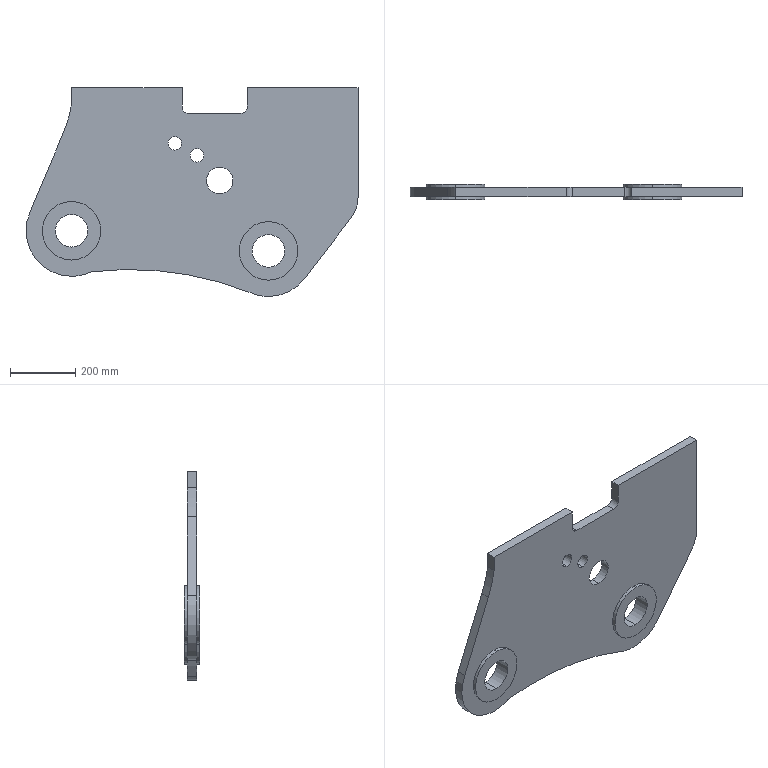Part | SolidWorks | features ICE 2, Extrusion 1 | 1 solid | 43 faces | box 1020 x 48 x 641.98 mm | volume 14814063 mm3 | cylinder 28 | plane 15 | commonest cylinder face diameters 180 x8 41.5 x4 100 x4 280 x4 40 x3 81.5 x2
STEP:
#1=CARTESIAN_POINT('',(2657.945,38.,-1778.762));
#2=VERTEX_POINT('',#1);
#3=CARTESIAN_POINT('',(2657.945,38.,-1958.762));
#4=VERTEX_POINT('',#3);
#5=CARTESIAN_POINT('',(2657.945,38.,-1868.762));
#6=DIRECTION('',(0.,1.,0.));
#7=DIRECTION('',(0.,0.,1.));
#8=AXIS2_PLACEMENT_3D('',#5,#6,#7);
#9=CIRCLE('',#8,90.);
#10=EDGE_CURVE('',#2,#4,#9,.T.);
#11=ORIENTED_EDGE('',*,*,#10,.F.);
#12=CARTESIAN_POINT('',(2657.945,28.,-1778.762));
#13=VERTEX_POINT('',#12);
#14=CARTESIAN_POINT('',(2657.945,38.,-1778.762));
#15=DIRECTION('',(0.,-1.,0.));
#16=VECTOR('',#15,1000.);
#17=LINE('',#14,#16);
#18=EDGE_CURVE('',#2,#13,#17,.T.);
#19=ORIENTED_EDGE('',*,*,#18,.T.);
#20=CARTESIAN_POINT('',(2657.945,28.,-1958.762));
#21=VERTEX_POINT('',#20);
#22=CARTESIAN_POINT('',(2657.945,28.,-1868.762));
#23=DIRECTION('',(0.,1.,0.));
#24=DIRECTION('',(0.,0.,1.));
#25=AXIS2_PLACEMENT_3D('',#22,#23,#24);
#26=CIRCLE('',#25,90.);
#27=EDGE_CURVE('',#13,#21,#26,.T.);
#28=ORIENTED_EDGE('',*,*,#27,.T.);
#29=CARTESIAN_POINT('',(2657.945,38.,-1958.762));
#30=DIRECTION('',(0.,-1.,0.));
#31=VECTOR('',#30,1000.);
#32=LINE('',#29,#31);
#33=EDGE_CURVE('',#4,#21,#32,.T.);
#34=ORIENTED_EDGE('',*,*,#33,.F.);
#35=EDGE_LOOP('',(#11,#19,#28,#34));
#36=FACE_OUTER_BOUND('',#35,.T.);
#37=CARTESIAN_POINT('',(2657.945,38.,-1868.762));
#38=DIRECTION('',(0.,-1.,0.));
#39=DIRECTION('',(0.,0.,-1.));
#40=AXIS2_PLACEMENT_3D('',#37,#38,#39);
#41=CYLINDRICAL_SURFACE('',#40,90.);
#42=ADVANCED_FACE('',(#36),#41,.T.);
#43=CARTESIAN_POINT('',(2657.945,-10.,-1918.762));
#44=VERTEX_POINT('',#43);
#45=CARTESIAN_POINT('',(2657.945,-10.,-1818.762));
#46=VERTEX_POINT('',#45);
#47=CARTESIAN_POINT('',(2657.945,-10.,-1868.762));
#48=DIRECTION('',(0.,1.,0.));
#49=DIRECTION('',(0.,0.,1.));
#50=AXIS2_PLACEMENT_3D('',#47,#48,#49);
#51=CIRCLE('',#50,50.);
#52=EDGE_CURVE('',#44,#46,#51,.T.);
#53=ORIENTED_EDGE('',*,*,#52,.F.);
#54=CARTESIAN_POINT('',(2657.945,38.,-1918.762));
#55=VERTEX_POINT('',#54);
#56=CARTESIAN_POINT('',(2657.945,-10.,-1918.762));
#57=DIRECTION('',(0.,1.,0.));
#58=VECTOR('',#57,1000.);
#59=LINE('',#56,#58);
#60=EDGE_CURVE('',#44,#55,#59,.T.);
#61=ORIENTED_EDGE('',*,*,#60,.T.);
#62=CARTESIAN_POINT('',(2657.945,38.,-1818.762));
#63=VERTEX_POINT('',#62);
#64=CARTESIAN_POINT('',(2657.945,38.,-1868.762));
#65=DIRECTION('',(0.,1.,0.));
#66=DIRECTION('',(0.,0.,1.));
#67=AXIS2_PLACEMENT_3D('',#64,#65,#66);
#68=CIRCLE('',#67,50.);
#69=EDGE_CURVE('',#55,#63,#68,.T.);
#70=ORIENTED_EDGE('',*,*,#69,.T.);
#71=CARTESIAN_POINT('',(2657.945,-10.,-1818.762));
#72=DIRECTION('',(0.,1.,0.));
#73=VECTOR('',#72,1000.);
#74=LINE('',#71,#73);
#75=EDGE_CURVE('',#46,#63,#74,.T.);
#76=ORIENTED_EDGE('',*,*,#75,.F.);
#77=EDGE_LOOP('',(#53,#61,#70,#76));
#78=FACE_OUTER_BOUND('',#77,.T.);
#79=CARTESIAN_POINT('',(2657.945,-10.,-1868.762));
#80=DIRECTION('',(0.,1.,0.));
#81=DIRECTION('',(0.,0.,1.));
#82=AXIS2_PLACEMENT_3D('',#79,#80,#81);
#83=CYLINDRICAL_SURFACE('',#82,50.);
#84=ADVANCED_FACE('',(#78),#83,.F.);
#85=CARTESIAN_POINT('',(2657.945,-10.,-1778.762));
#86=VERTEX_POINT('',#85);
#87=CARTESIAN_POINT('',(2657.945,-10.,-1958.762));
#88=VERTEX_POINT('',#87);
#89=CARTESIAN_POINT('',(2657.945,-10.,-1868.762));
#90=DIRECTION('',(0.,1.,0.));
#91=DIRECTION('',(0.,0.,1.));
#92=AXIS2_PLACEMENT_3D('',#89,#90,#91);
#93=CIRCLE('',#92,90.);
#94=EDGE_CURVE('',#86,#88,#93,.T.);
#95=ORIENTED_EDGE('',*,*,#94,.T.);
#96=CARTESIAN_POINT('',(2657.945,0.,-1958.762));
#97=VERTEX_POINT('',#96);
#98=CARTESIAN_POINT('',(2657.945,-10.,-1958.762));
#99=DIRECTION('',(0.,1.,0.));
#100=VECTOR('',#99,1000.);
#101=LINE('',#98,#100);
#102=EDGE_CURVE('',#88,#97,#101,.T.);
#103=ORIENTED_EDGE('',*,*,#102,.T.);
#104=CARTESIAN_POINT('',(2657.945,0.,-1778.762));
#105=VERTEX_POINT('',#104);
#106=CARTESIAN_POINT('',(2657.945,0.,-1868.762));
#107=DIRECTION('',(0.,1.,0.));
#108=DIRECTION('',(0.,0.,1.));
#109=AXIS2_PLACEMENT_3D('',#106,#107,#108);
#110=CIRCLE('',#109,90.);
#111=EDGE_CURVE('',#105,#97,#110,.T.);
#112=ORIENTED_EDGE('',*,*,#111,.F.);
#113=CARTESIAN_POINT('',(2657.945,-10.,-1778.762));
#114=DIRECTION('',(0.,1.,0.));
#115=VECTOR('',#114,1000.);
#116=LINE('',#113,#115);
#117=EDGE_CURVE('',#86,#105,#116,.T.);
#118=ORIENTED_EDGE('',*,*,#117,.F.);
#119=EDGE_LOOP('',(#95,#103,#112,#118));
#120=FACE_OUTER_BOUND('',#119,.T.);
#121=CARTESIAN_POINT('',(2657.945,-10.,-1868.762));
#122=DIRECTION('',(0.,1.,0.));
#123=DIRECTION('',(0.,0.,1.));
#124=AXIS2_PLACEMENT_3D('',#121,#122,#123);
#125=CYLINDRICAL_SURFACE('',#124,90.);
#126=ADVANCED_FACE('',(#120),#125,.T.);
#127=CARTESIAN_POINT('',(2052.944,38.,-1716.783));
#128=VERTEX_POINT('',#127);
#129=CARTESIAN_POINT('',(2052.944,38.,-1896.783));
#130=VERTEX_POINT('',#129);
#131=CARTESIAN_POINT('',(2052.944,38.,-1806.783));
#132=DIRECTION('',(0.,1.,0.));
#133=DIRECTION('',(0.,0.,1.));
#134=AXIS2_PLACEMENT_3D('',#131,#132,#133);
#135=CIRCLE('',#134,90.);
#136=EDGE_CURVE('',#128,#130,#135,.T.);
#137=ORIENTED_EDGE('',*,*,#136,.F.);
#138=CARTESIAN_POINT('',(2052.944,28.,-1716.783));
#139=VERTEX_POINT('',#138);
#140=CARTESIAN_POINT('',(2052.944,38.,-1716.783));
#141=DIRECTION('',(0.,-1.,0.));
#142=VECTOR('',#141,1000.);
#143=LINE('',#140,#142);
#144=EDGE_CURVE('',#128,#139,#143,.T.);
#145=ORIENTED_EDGE('',*,*,#144,.T.);
#146=CARTESIAN_POINT('',(2052.944,28.,-1896.783));
#147=VERTEX_POINT('',#146);
#148=CARTESIAN_POINT('',(2052.944,28.,-1806.783));
#149=DIRECTION('',(0.,1.,0.));
#150=DIRECTION('',(0.,0.,1.));
#151=AXIS2_PLACEMENT_3D('',#148,#149,#150);
#152=CIRCLE('',#151,90.);
#153=EDGE_CURVE('',#139,#147,#152,.T.);
#154=ORIENTED_EDGE('',*,*,#153,.T.);
#155=CARTESIAN_POINT('',(2052.944,38.,-1896.783));
#156=DIRECTION('',(0.,-1.,0.));
#157=VECTOR('',#156,1000.);
#158=LINE('',#155,#157);
#159=EDGE_CURVE('',#130,#147,#158,.T.);
#160=ORIENTED_EDGE('',*,*,#159,.F.);
#161=EDGE_LOOP('',(#137,#145,#154,#160));
#162=FACE_OUTER_BOUND('',#161,.T.);
#163=CARTESIAN_POINT('',(2052.944,38.,-1806.783));
#164=DIRECTION('',(0.,-1.,0.));
#165=DIRECTION('',(0.,0.,-1.));
#166=AXIS2_PLACEMENT_3D('',#163,#164,#165);
#167=CYLINDRICAL_SURFACE('',#166,90.);
#168=ADVANCED_FACE('',(#162),#167,.T.);
#169=CARTESIAN_POINT('',(2052.944,-10.,-1856.783));
#170=VERTEX_POINT('',#169);
#171=CARTESIAN_POINT('',(2052.944,-10.,-1756.783));
#172=VERTEX_POINT('',#171);
#173=CARTESIAN_POINT('',(2052.944,-10.,-1806.783));
#174=DIRECTION('',(0.,1.,0.));
#175=DIRECTION('',(0.,0.,1.));
#176=AXIS2_PLACEMENT_3D('',#173,#174,#175);
#177=CIRCLE('',#176,50.);
#178=EDGE_CURVE('',#170,#172,#177,.T.);
#179=ORIENTED_EDGE('',*,*,#178,.F.);
#180=CARTESIAN_POINT('',(2052.944,38.,-1856.783));
#181=VERTEX_POINT('',#180);
#182=CARTESIAN_POINT('',(2052.944,-10.,-1856.783));
#183=DIRECTION('',(0.,1.,0.));
#184=VECTOR('',#183,1000.);
#185=LINE('',#182,#184);
#186=EDGE_CURVE('',#170,#181,#185,.T.);
#187=ORIENTED_EDGE('',*,*,#186,.T.);
#188=CARTESIAN_POINT('',(2052.944,38.,-1756.783));
#189=VERTEX_POINT('',#188);
#190=CARTESIAN_POINT('',(2052.944,38.,-1806.783));
#191=DIRECTION('',(0.,1.,0.));
#192=DIRECTION('',(0.,0.,1.));
#193=AXIS2_PLACEMENT_3D('',#190,#191,#192);
#194=CIRCLE('',#193,50.);
#195=EDGE_CURVE('',#181,#189,#194,.T.);
#196=ORIENTED_EDGE('',*,*,#195,.T.);
#197=CARTESIAN_POINT('',(2052.944,-10.,-1756.783));
#198=DIRECTION('',(0.,1.,0.));
#199=VECTOR('',#198,1000.);
#200=LINE('',#197,#199);
#201=EDGE_CURVE('',#172,#189,#200,.T.);
#202=ORIENTED_EDGE('',*,*,#201,.F.);
#203=EDGE_LOOP('',(#179,#187,#196,#202));
#204=FACE_OUTER_BOUND('',#203,.T.);
#205=CARTESIAN_POINT('',(2052.944,-10.,-1806.783));
#206=DIRECTION('',(0.,1.,0.));
#207=DIRECTION('',(0.,0.,1.));
#208=AXIS2_PLACEMENT_3D('',#205,#206,#207);
#209=CYLINDRICAL_SURFACE('',#208,50.);
#210=ADVANCED_FACE('',(#204),#209,.F.);
#211=CARTESIAN_POINT('',(2052.944,-10.,-1716.783));
#212=VERTEX_POINT('',#211);
#213=CARTESIAN_POINT('',(2052.944,-10.,-1896.783));
#214=VERTEX_POINT('',#213);
#215=CARTESIAN_POINT('',(2052.944,-10.,-1806.783));
#216=DIRECTION('',(0.,1.,0.));
#217=DIRECTION('',(0.,0.,1.));
#218=AXIS2_PLACEMENT_3D('',#215,#216,#217);
#219=CIRCLE('',#218,90.);
#220=EDGE_CURVE('',#212,#214,#219,.T.);
#221=ORIENTED_EDGE('',*,*,#220,.T.);
#222=CARTESIAN_POINT('',(2052.944,0.,-1896.783));
#223=VERTEX_POINT('',#222);
#224=CARTESIAN_POINT('',(2052.944,-10.,-1896.783));
#225=DIRECTION('',(0.,1.,0.));
#226=VECTOR('',#225,1000.);
#227=LINE('',#224,#226);
#228=EDGE_CURVE('',#214,#223,#227,.T.);
#229=ORIENTED_EDGE('',*,*,#228,.T.);
#230=CARTESIAN_POINT('',(2052.944,0.,-1716.783));
#231=VERTEX_POINT('',#230);
#232=CARTESIAN_POINT('',(2052.944,0.,-1806.783));
#233=DIRECTION('',(0.,1.,0.));
#234=DIRECTION('',(0.,0.,1.));
#235=AXIS2_PLACEMENT_3D('',#232,#233,#234);
#236=CIRCLE('',#235,90.);
#237=EDGE_CURVE('',#231,#223,#236,.T.);
#238=ORIENTED_EDGE('',*,*,#237,.F.);
#239=CARTESIAN_POINT('',(2052.944,-10.,-1716.783));
#240=DIRECTION('',(0.,1.,0.));
#241=VECTOR('',#240,1000.);
#242=LINE('',#239,#241);
#243=EDGE_CURVE('',#212,#231,#242,.T.);
#244=ORIENTED_EDGE('',*,*,#243,.F.);
#245=EDGE_LOOP('',(#221,#229,#238,#244));
#246=FACE_OUTER_BOUND('',#245,.T.);
#247=CARTESIAN_POINT('',(2052.944,-10.,-1806.783));
#248=DIRECTION('',(0.,1.,0.));
#249=DIRECTION('',(0.,0.,1.));
#250=AXIS2_PLACEMENT_3D('',#247,#248,#249);
#251=CYLINDRICAL_SURFACE('',#250,90.);
#252=ADVANCED_FACE('',(#246),#251,.T.);
#253=CARTESIAN_POINT('',(2507.944,28.,-1693.533));
#254=VERTEX_POINT('',#253);
#255=CARTESIAN_POINT('',(2507.944,28.,-1612.033));
#256=VERTEX_POINT('',#255);
#257=CARTESIAN_POINT('',(2507.944,28.,-1652.783));
#258=DIRECTION('',(0.,1.,0.));
#259=DIRECTION('',(0.,0.,1.));
#260=AXIS2_PLACEMENT_3D('',#257,#258,#259);
#261=CIRCLE('',#260,40.75);
#262=EDGE_CURVE('',#254,#256,#261,.T.);
#263=ORIENTED_EDGE('',*,*,#262,.T.);
#264=CARTESIAN_POINT('',(2507.944,0.,-1612.033));
#265=VERTEX_POINT('',#264);
#266=CARTESIAN_POINT('',(2507.944,28.,-1612.033));
#267=DIRECTION('',(0.,-1.,0.));
#268=VECTOR('',#267,1000.);
#269=LINE('',#266,#268);
#270=EDGE_CURVE('',#256,#265,#269,.T.);
#271=ORIENTED_EDGE('',*,*,#270,.T.);
#272=CARTESIAN_POINT('',(2507.944,0.,-1693.533));
#273=VERTEX_POINT('',#272);
#274=CARTESIAN_POINT('',(2507.944,0.,-1652.783));
#275=DIRECTION('',(0.,1.,0.));
#276=DIRECTION('',(0.,0.,1.));
#277=AXIS2_PLACEMENT_3D('',#274,#275,#276);
#278=CIRCLE('',#277,40.75);
#279=EDGE_CURVE('',#273,#265,#278,.T.);
#280=ORIENTED_EDGE('',*,*,#279,.F.);
#281=CARTESIAN_POINT('',(2507.944,28.,-1693.533));
#282=DIRECTION('',(0.,-1.,0.));
#283=VECTOR('',#282,1000.);
#284=LINE('',#281,#283);
#285=EDGE_CURVE('',#254,#273,#284,.T.);
#286=ORIENTED_EDGE('',*,*,#285,.F.);
#287=EDGE_LOOP('',(#263,#271,#280,#286));
#288=FACE_OUTER_BOUND('',#287,.T.);
#289=CARTESIAN_POINT('',(2507.944,28.,-1652.783));
#290=DIRECTION('',(0.,-1.,0.));
#291=DIRECTION('',(0.,0.,-1.));
#292=AXIS2_PLACEMENT_3D('',#289,#290,#291);
#293=CYLINDRICAL_SURFACE('',#292,40.75);
#294=ADVANCED_FACE('',(#288),#293,.F.);
#295=CARTESIAN_POINT('',(2437.944,28.,-1596.033));
#296=VERTEX_POINT('',#295);
#297=CARTESIAN_POINT('',(2437.944,28.,-1554.533));
#298=VERTEX_POINT('',#297);
#299=CARTESIAN_POINT('',(2437.944,28.,-1575.283));
#300=DIRECTION('',(0.,1.,0.));
#301=DIRECTION('',(0.,0.,1.));
#302=AXIS2_PLACEMENT_3D('',#299,#300,#301);
#303=CIRCLE('',#302,20.75);
#304=EDGE_CURVE('',#296,#298,#303,.T.);
#305=ORIENTED_EDGE('',*,*,#304,.T.);
#306=CARTESIAN_POINT('',(2437.944,0.,-1554.533));
#307=VERTEX_POINT('',#306);
#308=CARTESIAN_POINT('',(2437.944,28.,-1554.533));
#309=DIRECTION('',(0.,-1.,0.));
#310=VECTOR('',#309,1000.);
#311=LINE('',#308,#310);
#312=EDGE_CURVE('',#298,#307,#311,.T.);
#313=ORIENTED_EDGE('',*,*,#312,.T.);
#314=CARTESIAN_POINT('',(2437.944,0.,-1596.033));
#315=VERTEX_POINT('',#314);
#316=CARTESIAN_POINT('',(2437.944,0.,-1575.283));
#317=DIRECTION('',(0.,1.,0.));
#318=DIRECTION('',(0.,0.,1.));
#319=AXIS2_PLACEMENT_3D('',#316,#317,#318);
#320=CIRCLE('',#319,20.75);
#321=EDGE_CURVE('',#315,#307,#320,.T.);
#322=ORIENTED_EDGE('',*,*,#321,.F.);
#323=CARTESIAN_POINT('',(2437.944,28.,-1596.033));
#324=DIRECTION('',(0.,-1.,0.));
#325=VECTOR('',#324,1000.);
#326=LINE('',#323,#325);
#327=EDGE_CURVE('',#296,#315,#326,.T.);
#328=ORIENTED_EDGE('',*,*,#327,.F.);
#329=EDGE_LOOP('',(#305,#313,#322,#328));
#330=FACE_OUTER_BOUND('',#329,.T.);
#331=CARTESIAN_POINT('',(2437.944,28.,-1575.283));
#332=DIRECTION('',(0.,-1.,0.));
#333=DIRECTION('',(0.,0.,-1.));
#334=AXIS2_PLACEMENT_3D('',#331,#332,#333);
#335=CYLINDRICAL_SURFACE('',#334,20.75);
#336=ADVANCED_FACE('',(#330),#335,.F.);
#337=CARTESIAN_POINT('',(2369.944,28.,-1559.033));
#338=VERTEX_POINT('',#337);
#339=CARTESIAN_POINT('',(2369.944,28.,-1517.533));
#340=VERTEX_POINT('',#339);
#341=CARTESIAN_POINT('',(2369.944,28.,-1538.283));
#342=DIRECTION('',(0.,1.,0.));
#343=DIRECTION('',(0.,0.,1.));
#344=AXIS2_PLACEMENT_3D('',#341,#342,#343);
#345=CIRCLE('',#344,20.75);
#346=EDGE_CURVE('',#338,#340,#345,.T.);
#347=ORIENTED_EDGE('',*,*,#346,.T.);
#348=CARTESIAN_POINT('',(2369.944,0.,-1517.533));
#349=VERTEX_POINT('',#348);
#350=CARTESIAN_POINT('',(2369.944,28.,-1517.533));
#351=DIRECTION('',(0.,-1.,0.));
#352=VECTOR('',#351,1000.);
#353=LINE('',#350,#352);
#354=EDGE_CURVE('',#340,#349,#353,.T.);
#355=ORIENTED_EDGE('',*,*,#354,.T.);
#356=CARTESIAN_POINT('',(2369.944,0.,-1559.033));
#357=VERTEX_POINT('',#356);
#358=CARTESIAN_POINT('',(2369.944,0.,-1538.283));
#359=DIRECTION('',(0.,1.,0.));
#360=DIRECTION('',(0.,0.,1.));
#361=AXIS2_PLACEMENT_3D('',#358,#359,#360);
#362=CIRCLE('',#361,20.75);
#363=EDGE_CURVE('',#357,#349,#362,.T.);
#364=ORIENTED_EDGE('',*,*,#363,.F.);
#365=CARTESIAN_POINT('',(2369.944,28.,-1559.033));
#366=DIRECTION('',(0.,-1.,0.));
#367=VECTOR('',#366,1000.);
#368=LINE('',#365,#367);
#369=EDGE_CURVE('',#338,#357,#368,.T.);
#370=ORIENTED_EDGE('',*,*,#369,.F.);
#371=EDGE_LOOP('',(#347,#355,#364,#370));
#372=FACE_OUTER_BOUND('',#371,.T.);
#373=CARTESIAN_POINT('',(2369.944,28.,-1538.283));
#374=DIRECTION('',(0.,-1.,0.));
#375=DIRECTION('',(0.,0.,-1.));
#376=AXIS2_PLACEMENT_3D('',#373,#374,#375);
#377=CYLINDRICAL_SURFACE('',#376,20.75);
#378=ADVANCED_FACE('',(#372),#377,.F.);
#379=CARTESIAN_POINT('',(2657.945,28.,-2008.762));
#380=VERTEX_POINT('',#379);
#381=CARTESIAN_POINT('',(2597.945,28.,-1995.254));
#382=VERTEX_POINT('',#381);
#383=CARTESIAN_POINT('',(2657.945,28.,-1868.762));
#384=DIRECTION('',(0.,1.,0.));
#385=DIRECTION('',(0.,0.,1.));
#386=AXIS2_PLACEMENT_3D('',#383,#384,#385);
#387=CIRCLE('',#386,140.);
#388=EDGE_CURVE('',#380,#382,#387,.T.);
#389=ORIENTED_EDGE('',*,*,#388,.F.);
#390=CARTESIAN_POINT('',(2657.945,0.,-2008.762));
#391=VERTEX_POINT('',#390);
#392=CARTESIAN_POINT('',(2657.945,28.,-2008.762));
#393=DIRECTION('',(0.,-1.,0.));
#394=VECTOR('',#393,1000.);
#395=LINE('',#392,#394);
#396=EDGE_CURVE('',#380,#391,#395,.T.);
#397=ORIENTED_EDGE('',*,*,#396,.T.);
#398=CARTESIAN_POINT('',(2597.945,0.,-1995.254));
#399=VERTEX_POINT('',#398);
#400=CARTESIAN_POINT('',(2657.945,0.,-1868.762));
#401=DIRECTION('',(0.,1.,0.));
#402=DIRECTION('',(0.,0.,1.));
#403=AXIS2_PLACEMENT_3D('',#400,#401,#402);
#404=CIRCLE('',#403,140.);
#405=EDGE_CURVE('',#391,#399,#404,.T.);
#406=ORIENTED_EDGE('',*,*,#405,.T.);
#407=CARTESIAN_POINT('',(2597.945,28.,-1995.254));
#408=DIRECTION('',(0.,-1.,0.));
#409=VECTOR('',#408,1000.);
#410=LINE('',#407,#409);
#411=EDGE_CURVE('',#382,#399,#410,.T.);
#412=ORIENTED_EDGE('',*,*,#411,.F.);
#413=EDGE_LOOP('',(#389,#397,#406,#412));
#414=FACE_OUTER_BOUND('',#413,.T.);
#415=CARTESIAN_POINT('',(2657.945,28.,-1868.762));
#416=DIRECTION('',(0.,-1.,0.));
#417=DIRECTION('',(0.,0.,-1.));
#418=AXIS2_PLACEMENT_3D('',#415,#416,#417);
#419=CYLINDRICAL_SURFACE('',#418,140.);
#420=ADVANCED_FACE('',(#414),#419,.T.);
#421=CARTESIAN_POINT('',(2052.944,28.,-1946.783));
#422=VERTEX_POINT('',#421);
#423=CARTESIAN_POINT('',(1925.701,28.,-1748.394));
#424=VERTEX_POINT('',#423);
#425=CARTESIAN_POINT('',(2052.944,28.,-1806.783));
#426=DIRECTION('',(0.,1.,0.));
#427=DIRECTION('',(0.,0.,1.));
#428=AXIS2_PLACEMENT_3D('',#425,#426,#427);
#429=CIRCLE('',#428,140.);
#430=EDGE_CURVE('',#422,#424,#429,.T.);
#431=ORIENTED_EDGE('',*,*,#430,.F.);
#432=CARTESIAN_POINT('',(2052.944,0.,-1946.783));
#433=VERTEX_POINT('',#432);
#434=CARTESIAN_POINT('',(2052.944,28.,-1946.783));
#435=DIRECTION('',(0.,-1.,0.));
#436=VECTOR('',#435,1000.);
#437=LINE('',#434,#436);
#438=EDGE_CURVE('',#422,#433,#437,.T.);
#439=ORIENTED_EDGE('',*,*,#438,.T.);
#440=CARTESIAN_POINT('',(1925.701,0.,-1748.394));
#441=VERTEX_POINT('',#440);
#442=CARTESIAN_POINT('',(2052.944,0.,-1806.783));
#443=DIRECTION('',(0.,1.,0.));
#444=DIRECTION('',(0.,0.,1.));
#445=AXIS2_PLACEMENT_3D('',#442,#443,#444);
#446=CIRCLE('',#445,140.);
#447=EDGE_CURVE('',#433,#441,#446,.T.);
#448=ORIENTED_EDGE('',*,*,#447,.T.);
#449=CARTESIAN_POINT('',(1925.701,28.,-1748.394));
#450=DIRECTION('',(0.,-1.,0.));
#451=VECTOR('',#450,1000.);
#452=LINE('',#449,#451);
#453=EDGE_CURVE('',#424,#441,#452,.T.);
#454=ORIENTED_EDGE('',*,*,#453,.F.);
#455=EDGE_LOOP('',(#431,#439,#448,#454));
#456=FACE_OUTER_BOUND('',#455,.T.);
#457=CARTESIAN_POINT('',(2052.944,28.,-1806.783));
#458=DIRECTION('',(0.,-1.,0.));
#459=DIRECTION('',(0.,0.,-1.));
#460=AXIS2_PLACEMENT_3D('',#457,#458,#459);
#461=CYLINDRICAL_SURFACE('',#460,140.);
#462=ADVANCED_FACE('',(#456),#461,.T.);
#463=CARTESIAN_POINT('',(2052.944,28.,-1806.783));
#464=DIRECTION('',(0.,1.,0.));
#465=DIRECTION('',(0.,0.,1.));
#466=AXIS2_PLACEMENT_3D('',#463,#464,#465);
#467=CIRCLE('',#466,90.);
#468=EDGE_CURVE('',#147,#139,#467,.T.);
#469=ORIENTED_EDGE('',*,*,#468,.F.);
#470=ORIENTED_EDGE('',*,*,#153,.F.);
#471=EDGE_LOOP('',(#469,#470));
#472=FACE_BOUND('',#471,.T.);
#473=ORIENTED_EDGE('',*,*,#304,.F.);
#474=CARTESIAN_POINT('',(2437.944,28.,-1575.283));
#475=DIRECTION('',(0.,1.,0.));
#476=DIRECTION('',(0.,0.,1.));
#477=AXIS2_PLACEMENT_3D('',#474,#475,#476);
#478=CIRCLE('',#477,20.75);
#479=EDGE_CURVE('',#298,#296,#478,.T.);
#480=ORIENTED_EDGE('',*,*,#479,.F.);
#481=EDGE_LOOP('',(#473,#480));
#482=FACE_BOUND('',#481,.T.);
#483=CARTESIAN_POINT('',(2116.599,28.,-1932.685));
#484=VERTEX_POINT('',#483);
#485=CARTESIAN_POINT('',(2110.666,28.,-1934.329));
#486=VERTEX_POINT('',#485);
#487=CARTESIAN_POINT('',(2118.912,28.,-1952.55));
#488=DIRECTION('',(0.,-1.,0.));
#489=DIRECTION('',(0.,0.,1.));
#490=AXIS2_PLACEMENT_3D('',#487,#488,#489);
#491=CIRCLE('',#490,20.);
#492=EDGE_CURVE('',#484,#486,#491,.T.);
#493=ORIENTED_EDGE('',*,*,#492,.T.);
#494=CARTESIAN_POINT('',(2052.944,28.,-1806.783));
#495=DIRECTION('',(0.,1.,0.));
#496=DIRECTION('',(0.,0.,1.));
#497=AXIS2_PLACEMENT_3D('',#494,#495,#496);
#498=CIRCLE('',#497,140.);
#499=EDGE_CURVE('',#486,#422,#498,.T.);
#500=ORIENTED_EDGE('',*,*,#499,.T.);
#501=ORIENTED_EDGE('',*,*,#430,.T.);
#502=CARTESIAN_POINT('',(2027.88,28.,-1505.832));
#503=VERTEX_POINT('',#502);
#504=CARTESIAN_POINT('',(1925.701,28.,-1748.394));
#505=DIRECTION('',(0.3882,0.,0.9216));
#506=VECTOR('',#505,1000.);
#507=LINE('',#504,#506);
#508=EDGE_CURVE('',#424,#503,#507,.T.);
#509=ORIENTED_EDGE('',*,*,#508,.T.);
#510=CARTESIAN_POINT('',(2052.944,28.,-1416.783));
#511=VERTEX_POINT('',#510);
#512=CARTESIAN_POINT('',(1684.134,28.,-1361.029));
#513=DIRECTION('',(0.,-1.,0.));
#514=DIRECTION('',(0.,0.,1.));
#515=AXIS2_PLACEMENT_3D('',#512,#513,#514);
#516=CIRCLE('',#515,373.);
#517=EDGE_CURVE('',#503,#511,#516,.T.);
#518=ORIENTED_EDGE('',*,*,#517,.T.);
#519=CARTESIAN_POINT('',(2052.944,28.,-1366.783));
#520=VERTEX_POINT('',#519);
#521=CARTESIAN_POINT('',(2052.944,28.,-1366.783));
#522=DIRECTION('',(0.,0.,1.));
#523=VECTOR('',#522,1000.);
#524=LINE('',#521,#523);
#525=EDGE_CURVE('',#511,#520,#524,.T.);
#526=ORIENTED_EDGE('',*,*,#525,.T.);
#527=CARTESIAN_POINT('',(2392.944,28.,-1366.783));
#528=VERTEX_POINT('',#527);
#529=CARTESIAN_POINT('',(2052.944,28.,-1366.783));
#530=DIRECTION('',(1.,0.,0.));
#531=VECTOR('',#530,1000.);
#532=LINE('',#529,#531);
#533=EDGE_CURVE('',#520,#528,#532,.T.);
#534=ORIENTED_EDGE('',*,*,#533,.T.);
#535=CARTESIAN_POINT('',(2392.944,28.,-1426.783));
#536=VERTEX_POINT('',#535);
#537=CARTESIAN_POINT('',(2392.944,28.,-1366.783));
#538=DIRECTION('',(0.,0.,-1.));
#539=VECTOR('',#538,1000.);
#540=LINE('',#537,#539);
#541=EDGE_CURVE('',#528,#536,#540,.T.);
#542=ORIENTED_EDGE('',*,*,#541,.T.);
#543=CARTESIAN_POINT('',(2412.944,28.,-1446.783));
#544=VERTEX_POINT('',#543);
#545=CARTESIAN_POINT('',(2412.944,28.,-1426.783));
#546=DIRECTION('',(0.,-1.,0.));
#547=DIRECTION('',(0.,0.,1.));
#548=AXIS2_PLACEMENT_3D('',#545,#546,#547);
#549=CIRCLE('',#548,20.);
#550=EDGE_CURVE('',#536,#544,#549,.T.);
#551=ORIENTED_EDGE('',*,*,#550,.T.);
#552=CARTESIAN_POINT('',(2572.944,28.,-1446.783));
#553=VERTEX_POINT('',#552);
#554=CARTESIAN_POINT('',(2412.944,28.,-1446.783));
#555=DIRECTION('',(1.,0.,0.));
#556=VECTOR('',#555,1000.);
#557=LINE('',#554,#556);
#558=EDGE_CURVE('',#544,#553,#557,.T.);
#559=ORIENTED_EDGE('',*,*,#558,.T.);
#560=CARTESIAN_POINT('',(2592.944,28.,-1426.783));
#561=VERTEX_POINT('',#560);
#562=CARTESIAN_POINT('',(2572.944,28.,-1426.783));
#563=DIRECTION('',(0.,-1.,0.));
#564=DIRECTION('',(0.,0.,1.));
#565=AXIS2_PLACEMENT_3D('',#562,#563,#564);
#566=CIRCLE('',#565,20.);
#567=EDGE_CURVE('',#553,#561,#566,.T.);
#568=ORIENTED_EDGE('',*,*,#567,.T.);
#569=CARTESIAN_POINT('',(2592.944,28.,-1366.783));
#570=VERTEX_POINT('',#569);
#571=CARTESIAN_POINT('',(2592.944,28.,-1366.783));
#572=DIRECTION('',(0.,0.,1.));
#573=VECTOR('',#572,1000.);
#574=LINE('',#571,#573);
#575=EDGE_CURVE('',#561,#570,#574,.T.);
#576=ORIENTED_EDGE('',*,*,#575,.T.);
#577=CARTESIAN_POINT('',(2932.944,28.,-1366.783));
#578=VERTEX_POINT('',#577);
#579=CARTESIAN_POINT('',(2592.944,28.,-1366.783));
#580=DIRECTION('',(1.,0.,0.));
#581=VECTOR('',#580,1000.);
#582=LINE('',#579,#581);
#583=EDGE_CURVE('',#570,#578,#582,.T.);
#584=ORIENTED_EDGE('',*,*,#583,.T.);
#585=CARTESIAN_POINT('',(2932.944,28.,-1705.999));
#586=VERTEX_POINT('',#585);
#587=CARTESIAN_POINT('',(2932.944,28.,-1366.783));
#588=DIRECTION('',(0.,0.,-1.));
#589=VECTOR('',#588,1000.);
#590=LINE('',#587,#589);
#591=EDGE_CURVE('',#578,#586,#590,.T.);
#592=ORIENTED_EDGE('',*,*,#591,.T.);
#593=CARTESIAN_POINT('',(2912.343,28.,-1766.792));
#594=VERTEX_POINT('',#593);
#595=CARTESIAN_POINT('',(2832.944,28.,-1705.999));
#596=DIRECTION('',(0.,1.,0.));
#597=DIRECTION('',(0.,0.,1.));
#598=AXIS2_PLACEMENT_3D('',#595,#596,#597);
#599=CIRCLE('',#598,100.);
#600=EDGE_CURVE('',#586,#594,#599,.T.);
#601=ORIENTED_EDGE('',*,*,#600,.T.);
#602=CARTESIAN_POINT('',(2769.103,28.,-1953.872));
#603=VERTEX_POINT('',#602);
#604=CARTESIAN_POINT('',(2769.103,28.,-1953.872));
#605=DIRECTION('',(-0.6079,0.,-0.794));
#606=VECTOR('',#605,1000.);
#607=LINE('',#604,#606);
#608=EDGE_CURVE('',#594,#603,#607,.T.);
#609=ORIENTED_EDGE('',*,*,#608,.T.);
#610=CARTESIAN_POINT('',(2657.945,28.,-1868.762));
#611=DIRECTION('',(0.,1.,0.));
#612=DIRECTION('',(0.,0.,1.));
#613=AXIS2_PLACEMENT_3D('',#610,#611,#612);
#614=CIRCLE('',#613,140.);
#615=EDGE_CURVE('',#603,#380,#614,.T.);
#616=ORIENTED_EDGE('',*,*,#615,.T.);
#617=ORIENTED_EDGE('',*,*,#388,.T.);
#618=CARTESIAN_POINT('',(2232.236,28.,-2925.878));
#619=DIRECTION('',(0.,-1.,0.));
#620=DIRECTION('',(0.,0.,1.));
#621=AXIS2_PLACEMENT_3D('',#618,#619,#620);
#622=CIRCLE('',#621,999.903);
#623=EDGE_CURVE('',#382,#484,#622,.T.);
#624=ORIENTED_EDGE('',*,*,#623,.T.);
#625=EDGE_LOOP('',(#493,#500,#501,#509,#518,#526,#534,#542,#551,#559,#568,#576,#584,#592,#601,#609,#616,#617,#624));
#626=FACE_OUTER_BOUND('',#625,.T.);
#627=ORIENTED_EDGE('',*,*,#346,.F.);
#628=CARTESIAN_POINT('',(2369.944,28.,-1538.283));
#629=DIRECTION('',(0.,1.,0.));
#630=DIRECTION('',(0.,0.,1.));
#631=AXIS2_PLACEMENT_3D('',#628,#629,#630);
#632=CIRCLE('',#631,20.75);
#633=EDGE_CURVE('',#340,#338,#632,.T.);
#634=ORIENTED_EDGE('',*,*,#633,.F.);
#635=EDGE_LOOP('',(#627,#634));
#636=FACE_BOUND('',#635,.T.);
#637=ORIENTED_EDGE('',*,*,#262,.F.);
#638=CARTESIAN_POINT('',(2507.944,28.,-1652.783));
#639=DIRECTION('',(0.,1.,0.));
#640=DIRECTION('',(0.,0.,1.));
#641=AXIS2_PLACEMENT_3D('',#638,#639,#640);
#642=CIRCLE('',#641,40.75);
#643=EDGE_CURVE('',#256,#254,#642,.T.);
#644=ORIENTED_EDGE('',*,*,#643,.F.);
#645=EDGE_LOOP('',(#637,#644));
#646=FACE_BOUND('',#645,.T.);
#647=CARTESIAN_POINT('',(2657.945,28.,-1868.762));
#648=DIRECTION('',(0.,1.,0.));
#649=DIRECTION('',(0.,0.,1.));
#650=AXIS2_PLACEMENT_3D('',#647,#648,#649);
#651=CIRCLE('',#650,90.);
#652=EDGE_CURVE('',#21,#13,#651,.T.);
#653=ORIENTED_EDGE('',*,*,#652,.F.);
#654=ORIENTED_EDGE('',*,*,#27,.F.);
#655=EDGE_LOOP('',(#653,#654));
#656=FACE_BOUND('',#655,.T.);
#657=CARTESIAN_POINT('',(2118.912,28.,-1952.55));
#658=DIRECTION('',(0.,1.,0.));
#659=DIRECTION('',(0.,0.,1.));
#660=AXIS2_PLACEMENT_3D('',#657,#658,#659);
#661=PLANE('',#660);
#662=ADVANCED_FACE('',(#472,#482,#626,#636,#646,#656),#661,.T.);
#663=CARTESIAN_POINT('',(2116.599,0.,-1932.685));
#664=VERTEX_POINT('',#663);
#665=CARTESIAN_POINT('',(2110.666,0.,-1934.329));
#666=VERTEX_POINT('',#665);
#667=CARTESIAN_POINT('',(2118.912,0.,-1952.55));
#668=DIRECTION('',(0.,-1.,0.));
#669=DIRECTION('',(0.,0.,1.));
#670=AXIS2_PLACEMENT_3D('',#667,#668,#669);
#671=CIRCLE('',#670,20.);
#672=EDGE_CURVE('',#664,#666,#671,.T.);
#673=ORIENTED_EDGE('',*,*,#672,.F.);
#674=CARTESIAN_POINT('',(2232.236,0.,-2925.878));
#675=DIRECTION('',(0.,-1.,0.));
#676=DIRECTION('',(0.,0.,1.));
#677=AXIS2_PLACEMENT_3D('',#674,#675,#676);
#678=CIRCLE('',#677,999.903);
#679=EDGE_CURVE('',#399,#664,#678,.T.);
#680=ORIENTED_EDGE('',*,*,#679,.F.);
#681=ORIENTED_EDGE('',*,*,#405,.F.);
#682=CARTESIAN_POINT('',(2769.103,0.,-1953.872));
#683=VERTEX_POINT('',#682);
#684=CARTESIAN_POINT('',(2657.945,0.,-1868.762));
#685=DIRECTION('',(0.,1.,0.));
#686=DIRECTION('',(0.,0.,1.));
#687=AXIS2_PLACEMENT_3D('',#684,#685,#686);
#688=CIRCLE('',#687,140.);
#689=EDGE_CURVE('',#683,#391,#688,.T.);
#690=ORIENTED_EDGE('',*,*,#689,.F.);
#691=CARTESIAN_POINT('',(2912.343,0.,-1766.792));
#692=VERTEX_POINT('',#691);
#693=CARTESIAN_POINT('',(2769.103,0.,-1953.872));
#694=DIRECTION('',(-0.6079,0.,-0.794));
#695=VECTOR('',#694,1000.);
#696=LINE('',#693,#695);
#697=EDGE_CURVE('',#692,#683,#696,.T.);
#698=ORIENTED_EDGE('',*,*,#697,.F.);
#699=CARTESIAN_POINT('',(2932.944,0.,-1705.999));
#700=VERTEX_POINT('',#699);
#701=CARTESIAN_POINT('',(2832.944,0.,-1705.999));
#702=DIRECTION('',(0.,1.,0.));
#703=DIRECTION('',(0.,0.,1.));
#704=AXIS2_PLACEMENT_3D('',#701,#702,#703);
#705=CIRCLE('',#704,100.);
#706=EDGE_CURVE('',#700,#692,#705,.T.);
#707=ORIENTED_EDGE('',*,*,#706,.F.);
#708=CARTESIAN_POINT('',(2932.944,0.,-1366.783));
#709=VERTEX_POINT('',#708);
#710=CARTESIAN_POINT('',(2932.944,0.,-1366.783));
#711=DIRECTION('',(0.,0.,-1.));
#712=VECTOR('',#711,1000.);
#713=LINE('',#710,#712);
#714=EDGE_CURVE('',#709,#700,#713,.T.);
#715=ORIENTED_EDGE('',*,*,#714,.F.);
#716=CARTESIAN_POINT('',(2592.944,0.,-1366.783));
#717=VERTEX_POINT('',#716);
#718=CARTESIAN_POINT('',(2592.944,0.,-1366.783));
#719=DIRECTION('',(1.,0.,0.));
#720=VECTOR('',#719,1000.);
#721=LINE('',#718,#720);
#722=EDGE_CURVE('',#717,#709,#721,.T.);
#723=ORIENTED_EDGE('',*,*,#722,.F.);
#724=CARTESIAN_POINT('',(2592.944,0.,-1426.783));
#725=VERTEX_POINT('',#724);
#726=CARTESIAN_POINT('',(2592.944,0.,-1366.783));
#727=DIRECTION('',(0.,0.,1.));
#728=VECTOR('',#727,1000.);
#729=LINE('',#726,#728);
#730=EDGE_CURVE('',#725,#717,#729,.T.);
#731=ORIENTED_EDGE('',*,*,#730,.F.);
#732=CARTESIAN_POINT('',(2572.944,0.,-1446.783));
#733=VERTEX_POINT('',#732);
#734=CARTESIAN_POINT('',(2572.944,0.,-1426.783));
#735=DIRECTION('',(0.,-1.,0.));
#736=DIRECTION('',(0.,0.,1.));
#737=AXIS2_PLACEMENT_3D('',#734,#735,#736);
#738=CIRCLE('',#737,20.);
#739=EDGE_CURVE('',#733,#725,#738,.T.);
#740=ORIENTED_EDGE('',*,*,#739,.F.);
#741=CARTESIAN_POINT('',(2412.944,0.,-1446.783));
#742=VERTEX_POINT('',#741);
#743=CARTESIAN_POINT('',(2412.944,0.,-1446.783));
#744=DIRECTION('',(1.,0.,0.));
#745=VECTOR('',#744,1000.);
#746=LINE('',#743,#745);
#747=EDGE_CURVE('',#742,#733,#746,.T.);
#748=ORIENTED_EDGE('',*,*,#747,.F.);
#749=CARTESIAN_POINT('',(2392.944,0.,-1426.783));
#750=VERTEX_POINT('',#749);
#751=CARTESIAN_POINT('',(2412.944,0.,-1426.783));
#752=DIRECTION('',(0.,-1.,0.));
#753=DIRECTION('',(0.,0.,1.));
#754=AXIS2_PLACEMENT_3D('',#751,#752,#753);
#755=CIRCLE('',#754,20.);
#756=EDGE_CURVE('',#750,#742,#755,.T.);
#757=ORIENTED_EDGE('',*,*,#756,.F.);
#758=CARTESIAN_POINT('',(2392.944,0.,-1366.783));
#759=VERTEX_POINT('',#758);
#760=CARTESIAN_POINT('',(2392.944,0.,-1366.783));
#761=DIRECTION('',(0.,0.,-1.));
#762=VECTOR('',#761,1000.);
#763=LINE('',#760,#762);
#764=EDGE_CURVE('',#759,#750,#763,.T.);
#765=ORIENTED_EDGE('',*,*,#764,.F.);
#766=CARTESIAN_POINT('',(2052.944,0.,-1366.783));
#767=VERTEX_POINT('',#766);
#768=CARTESIAN_POINT('',(2052.944,0.,-1366.783));
#769=DIRECTION('',(1.,0.,0.));
#770=VECTOR('',#769,1000.);
#771=LINE('',#768,#770);
#772=EDGE_CURVE('',#767,#759,#771,.T.);
#773=ORIENTED_EDGE('',*,*,#772,.F.);
#774=CARTESIAN_POINT('',(2052.944,0.,-1416.783));
#775=VERTEX_POINT('',#774);
#776=CARTESIAN_POINT('',(2052.944,0.,-1366.783));
#777=DIRECTION('',(0.,0.,1.));
#778=VECTOR('',#777,1000.);
#779=LINE('',#776,#778);
#780=EDGE_CURVE('',#775,#767,#779,.T.);
#781=ORIENTED_EDGE('',*,*,#780,.F.);
#782=CARTESIAN_POINT('',(2027.88,0.,-1505.832));
#783=VERTEX_POINT('',#782);
#784=CARTESIAN_POINT('',(1684.134,0.,-1361.029));
#785=DIRECTION('',(0.,-1.,0.));
#786=DIRECTION('',(0.,0.,1.));
#787=AXIS2_PLACEMENT_3D('',#784,#785,#786);
#788=CIRCLE('',#787,373.);
#789=EDGE_CURVE('',#783,#775,#788,.T.);
#790=ORIENTED_EDGE('',*,*,#789,.F.);
#791=CARTESIAN_POINT('',(1925.701,0.,-1748.394));
#792=DIRECTION('',(0.3882,0.,0.9216));
#793=VECTOR('',#792,1000.);
#794=LINE('',#791,#793);
#795=EDGE_CURVE('',#441,#783,#794,.T.);
#796=ORIENTED_EDGE('',*,*,#795,.F.);
#797=ORIENTED_EDGE('',*,*,#447,.F.);
#798=CARTESIAN_POINT('',(2052.944,0.,-1806.783));
#799=DIRECTION('',(0.,1.,0.));
#800=DIRECTION('',(0.,0.,1.));
#801=AXIS2_PLACEMENT_3D('',#798,#799,#800);
#802=CIRCLE('',#801,140.);
#803=EDGE_CURVE('',#666,#433,#802,.T.);
#804=ORIENTED_EDGE('',*,*,#803,.F.);
#805=EDGE_LOOP('',(#673,#680,#681,#690,#698,#707,#715,#723,#731,#740,#748,#757,#765,#773,#781,#790,#796,#797,#804));
#806=FACE_OUTER_BOUND('',#805,.T.);
#807=ORIENTED_EDGE('',*,*,#363,.T.);
#808=CARTESIAN_POINT('',(2369.944,0.,-1538.283));
#809=DIRECTION('',(0.,1.,0.));
#810=DIRECTION('',(0.,0.,1.));
#811=AXIS2_PLACEMENT_3D('',#808,#809,#810);
#812=CIRCLE('',#811,20.75);
#813=EDGE_CURVE('',#349,#357,#812,.T.);
#814=ORIENTED_EDGE('',*,*,#813,.T.);
#815=EDGE_LOOP('',(#807,#814));
#816=FACE_BOUND('',#815,.T.);
#817=ORIENTED_EDGE('',*,*,#321,.T.);
#818=CARTESIAN_POINT('',(2437.944,0.,-1575.283));
#819=DIRECTION('',(0.,1.,0.));
#820=DIRECTION('',(0.,0.,1.));
#821=AXIS2_PLACEMENT_3D('',#818,#819,#820);
#822=CIRCLE('',#821,20.75);
#823=EDGE_CURVE('',#307,#315,#822,.T.);
#824=ORIENTED_EDGE('',*,*,#823,.T.);
#825=EDGE_LOOP('',(#817,#824));
#826=FACE_BOUND('',#825,.T.);
#827=ORIENTED_EDGE('',*,*,#237,.T.);
#828=CARTESIAN_POINT('',(2052.944,0.,-1806.783));
#829=DIRECTION('',(0.,1.,0.));
#830=DIRECTION('',(0.,0.,1.));
#831=AXIS2_PLACEMENT_3D('',#828,#829,#830);
#832=CIRCLE('',#831,90.);
#833=EDGE_CURVE('',#223,#231,#832,.T.);
#834=ORIENTED_EDGE('',*,*,#833,.T.);
#835=EDGE_LOOP('',(#827,#834));
#836=FACE_BOUND('',#835,.T.);
#837=ORIENTED_EDGE('',*,*,#111,.T.);
#838=CARTESIAN_POINT('',(2657.945,0.,-1868.762));
#839=DIRECTION('',(0.,1.,0.));
#840=DIRECTION('',(0.,0.,1.));
#841=AXIS2_PLACEMENT_3D('',#838,#839,#840);
#842=CIRCLE('',#841,90.);
#843=EDGE_CURVE('',#97,#105,#842,.T.);
#844=ORIENTED_EDGE('',*,*,#843,.T.);
#845=EDGE_LOOP('',(#837,#844));
#846=FACE_BOUND('',#845,.T.);
#847=ORIENTED_EDGE('',*,*,#279,.T.);
#848=CARTESIAN_POINT('',(2507.944,0.,-1652.783));
#849=DIRECTION('',(0.,1.,0.));
#850=DIRECTION('',(0.,0.,1.));
#851=AXIS2_PLACEMENT_3D('',#848,#849,#850);
#852=CIRCLE('',#851,40.75);
#853=EDGE_CURVE('',#265,#273,#852,.T.);
#854=ORIENTED_EDGE('',*,*,#853,.T.);
#855=EDGE_LOOP('',(#847,#854));
#856=FACE_BOUND('',#855,.T.);
#857=CARTESIAN_POINT('',(2118.912,0.,-1952.55));
#858=DIRECTION('',(0.,1.,0.));
#859=DIRECTION('',(0.,0.,1.));
#860=AXIS2_PLACEMENT_3D('',#857,#858,#859);
#861=PLANE('',#860);
#862=ADVANCED_FACE('',(#806,#816,#826,#836,#846,#856),#861,.F.);
#863=ORIENTED_EDGE('',*,*,#672,.T.);
#864=CARTESIAN_POINT('',(2110.666,28.,-1934.329));
#865=DIRECTION('',(0.,-1.,0.));
#866=VECTOR('',#865,1000.);
#867=LINE('',#864,#866);
#868=EDGE_CURVE('',#486,#666,#867,.T.);
#869=ORIENTED_EDGE('',*,*,#868,.F.);
#870=ORIENTED_EDGE('',*,*,#492,.F.);
#871=CARTESIAN_POINT('',(2116.599,28.,-1932.685));
#872=DIRECTION('',(0.,-1.,0.));
#873=VECTOR('',#872,1000.);
#874=LINE('',#871,#873);
#875=EDGE_CURVE('',#484,#664,#874,.T.);
#876=ORIENTED_EDGE('',*,*,#875,.T.);
#877=EDGE_LOOP('',(#863,#869,#870,#876));
#878=FACE_OUTER_BOUND('',#877,.T.);
#879=CARTESIAN_POINT('',(2118.912,28.,-1952.55));
#880=DIRECTION('',(0.,-1.,0.));
#881=DIRECTION('',(0.,0.,-1.));
#882=AXIS2_PLACEMENT_3D('',#879,#880,#881);
#883=CYLINDRICAL_SURFACE('',#882,20.);
#884=ADVANCED_FACE('',(#878),#883,.F.);
#885=ORIENTED_EDGE('',*,*,#438,.F.);
#886=ORIENTED_EDGE('',*,*,#499,.F.);
#887=ORIENTED_EDGE('',*,*,#868,.T.);
#888=ORIENTED_EDGE('',*,*,#803,.T.);
#889=EDGE_LOOP('',(#885,#886,#887,#888));
#890=FACE_OUTER_BOUND('',#889,.T.);
#891=CARTESIAN_POINT('',(2052.944,28.,-1806.783));
#892=DIRECTION('',(0.,-1.,0.));
#893=DIRECTION('',(0.,0.,-1.));
#894=AXIS2_PLACEMENT_3D('',#891,#892,#893);
#895=CYLINDRICAL_SURFACE('',#894,140.);
#896=ADVANCED_FACE('',(#890),#895,.T.);
#897=ORIENTED_EDGE('',*,*,#795,.T.);
#898=CARTESIAN_POINT('',(2027.88,28.,-1505.832));
#899=DIRECTION('',(0.,-1.,0.));
#900=VECTOR('',#899,1000.);
#901=LINE('',#898,#900);
#902=EDGE_CURVE('',#503,#783,#901,.T.);
#903=ORIENTED_EDGE('',*,*,#902,.F.);
#904=ORIENTED_EDGE('',*,*,#508,.F.);
#905=ORIENTED_EDGE('',*,*,#453,.T.);
#906=EDGE_LOOP('',(#897,#903,#904,#905));
#907=FACE_OUTER_BOUND('',#906,.T.);
#908=CARTESIAN_POINT('',(1925.701,28.,-1748.394));
#909=DIRECTION('',(0.9216,0.,-0.3882));
#910=DIRECTION('',(-0.3882,0.,-0.9216));
#911=AXIS2_PLACEMENT_3D('',#908,#909,#910);
#912=PLANE('',#911);
#913=ADVANCED_FACE('',(#907),#912,.F.);
#914=ORIENTED_EDGE('',*,*,#789,.T.);
#915=CARTESIAN_POINT('',(2052.944,28.,-1416.783));
#916=DIRECTION('',(0.,-1.,0.));
#917=VECTOR('',#916,1000.);
#918=LINE('',#915,#917);
#919=EDGE_CURVE('',#511,#775,#918,.T.);
#920=ORIENTED_EDGE('',*,*,#919,.F.);
#921=ORIENTED_EDGE('',*,*,#517,.F.);
#922=ORIENTED_EDGE('',*,*,#902,.T.);
#923=EDGE_LOOP('',(#914,#920,#921,#922));
#924=FACE_OUTER_BOUND('',#923,.T.);
#925=CARTESIAN_POINT('',(1684.134,28.,-1361.029));
#926=DIRECTION('',(0.,-1.,0.));
#927=DIRECTION('',(0.,0.,-1.));
#928=AXIS2_PLACEMENT_3D('',#925,#926,#927);
#929=CYLINDRICAL_SURFACE('',#928,373.);
#930=ADVANCED_FACE('',(#924),#929,.F.);
#931=ORIENTED_EDGE('',*,*,#780,.T.);
#932=CARTESIAN_POINT('',(2052.944,28.,-1366.783));
#933=DIRECTION('',(0.,-1.,0.));
#934=VECTOR('',#933,1000.);
#935=LINE('',#932,#934);
#936=EDGE_CURVE('',#520,#767,#935,.T.);
#937=ORIENTED_EDGE('',*,*,#936,.F.);
#938=ORIENTED_EDGE('',*,*,#525,.F.);
#939=ORIENTED_EDGE('',*,*,#919,.T.);
#940=EDGE_LOOP('',(#931,#937,#938,#939));
#941=FACE_OUTER_BOUND('',#940,.T.);
#942=CARTESIAN_POINT('',(2052.944,28.,-1366.783));
#943=DIRECTION('',(1.,0.,0.));
#944=DIRECTION('',(0.,0.,-1.));
#945=AXIS2_PLACEMENT_3D('',#942,#943,#944);
#946=PLANE('',#945);
#947=ADVANCED_FACE('',(#941),#946,.F.);
#948=ORIENTED_EDGE('',*,*,#772,.T.);
#949=CARTESIAN_POINT('',(2392.944,28.,-1366.783));
#950=DIRECTION('',(0.,-1.,0.));
#951=VECTOR('',#950,1000.);
#952=LINE('',#949,#951);
#953=EDGE_CURVE('',#528,#759,#952,.T.);
#954=ORIENTED_EDGE('',*,*,#953,.F.);
#955=ORIENTED_EDGE('',*,*,#533,.F.);
#956=ORIENTED_EDGE('',*,*,#936,.T.);
#957=EDGE_LOOP('',(#948,#954,#955,#956));
#958=FACE_OUTER_BOUND('',#957,.T.);
#959=CARTESIAN_POINT('',(2052.944,28.,-1366.783));
#960=DIRECTION('',(0.,0.,-1.));
#961=DIRECTION('',(-1.,0.,0.));
#962=AXIS2_PLACEMENT_3D('',#959,#960,#961);
#963=PLANE('',#962);
#964=ADVANCED_FACE('',(#958),#963,.F.);
#965=ORIENTED_EDGE('',*,*,#764,.T.);
#966=CARTESIAN_POINT('',(2392.944,28.,-1426.783));
#967=DIRECTION('',(0.,-1.,0.));
#968=VECTOR('',#967,1000.);
#969=LINE('',#966,#968);
#970=EDGE_CURVE('',#536,#750,#969,.T.);
#971=ORIENTED_EDGE('',*,*,#970,.F.);
#972=ORIENTED_EDGE('',*,*,#541,.F.);
#973=ORIENTED_EDGE('',*,*,#953,.T.);
#974=EDGE_LOOP('',(#965,#971,#972,#973));
#975=FACE_OUTER_BOUND('',#974,.T.);
#976=CARTESIAN_POINT('',(2392.944,28.,-1366.783));
#977=DIRECTION('',(-1.,0.,0.));
#978=DIRECTION('',(0.,0.,1.));
#979=AXIS2_PLACEMENT_3D('',#976,#977,#978);
#980=PLANE('',#979);
#981=ADVANCED_FACE('',(#975),#980,.F.);
#982=ORIENTED_EDGE('',*,*,#756,.T.);
#983=CARTESIAN_POINT('',(2412.944,28.,-1446.783));
#984=DIRECTION('',(0.,-1.,0.));
#985=VECTOR('',#984,1000.);
#986=LINE('',#983,#985);
#987=EDGE_CURVE('',#544,#742,#986,.T.);
#988=ORIENTED_EDGE('',*,*,#987,.F.);
#989=ORIENTED_EDGE('',*,*,#550,.F.);
#990=ORIENTED_EDGE('',*,*,#970,.T.);
#991=EDGE_LOOP('',(#982,#988,#989,#990));
#992=FACE_OUTER_BOUND('',#991,.T.);
#993=CARTESIAN_POINT('',(2412.944,28.,-1426.783));
#994=DIRECTION('',(0.,-1.,0.));
#995=DIRECTION('',(0.,0.,-1.));
#996=AXIS2_PLACEMENT_3D('',#993,#994,#995);
#997=CYLINDRICAL_SURFACE('',#996,20.);
#998=ADVANCED_FACE('',(#992),#997,.F.);
#999=ORIENTED_EDGE('',*,*,#747,.T.);
#1000=CARTESIAN_POINT('',(2572.944,28.,-1446.783));
#1001=DIRECTION('',(0.,-1.,0.));
#1002=VECTOR('',#1001,1000.);
#1003=LINE('',#1000,#1002);
#1004=EDGE_CURVE('',#553,#733,#1003,.T.);
#1005=ORIENTED_EDGE('',*,*,#1004,.F.);
#1006=ORIENTED_EDGE('',*,*,#558,.F.);
#1007=ORIENTED_EDGE('',*,*,#987,.T.);
#1008=EDGE_LOOP('',(#999,#1005,#1006,#1007));
#1009=FACE_OUTER_BOUND('',#1008,.T.);
#1010=CARTESIAN_POINT('',(2412.944,28.,-1446.783));
#1011=DIRECTION('',(0.,0.,-1.));
#1012=DIRECTION('',(-1.,0.,0.));
#1013=AXIS2_PLACEMENT_3D('',#1010,#1011,#1012);
#1014=PLANE('',#1013);
#1015=ADVANCED_FACE('',(#1009),#1014,.F.);
#1016=ORIENTED_EDGE('',*,*,#739,.T.);
#1017=CARTESIAN_POINT('',(2592.944,28.,-1426.783));
#1018=DIRECTION('',(0.,-1.,0.));
#1019=VECTOR('',#1018,1000.);
#1020=LINE('',#1017,#1019);
#1021=EDGE_CURVE('',#561,#725,#1020,.T.);
#1022=ORIENTED_EDGE('',*,*,#1021,.F.);
#1023=ORIENTED_EDGE('',*,*,#567,.F.);
#1024=ORIENTED_EDGE('',*,*,#1004,.T.);
#1025=EDGE_LOOP('',(#1016,#1022,#1023,#1024));
#1026=FACE_OUTER_BOUND('',#1025,.T.);
#1027=CARTESIAN_POINT('',(2572.944,28.,-1426.783));
#1028=DIRECTION('',(0.,-1.,0.));
#1029=DIRECTION('',(0.,0.,-1.));
#1030=AXIS2_PLACEMENT_3D('',#1027,#1028,#1029);
#1031=CYLINDRICAL_SURFACE('',#1030,20.);
#1032=ADVANCED_FACE('',(#1026),#1031,.F.);
#1033=ORIENTED_EDGE('',*,*,#730,.T.);
#1034=CARTESIAN_POINT('',(2592.944,28.,-1366.783));
#1035=DIRECTION('',(0.,-1.,0.));
#1036=VECTOR('',#1035,1000.);
#1037=LINE('',#1034,#1036);
#1038=EDGE_CURVE('',#570,#717,#1037,.T.);
#1039=ORIENTED_EDGE('',*,*,#1038,.F.);
#1040=ORIENTED_EDGE('',*,*,#575,.F.);
#1041=ORIENTED_EDGE('',*,*,#1021,.T.);
#1042=EDGE_LOOP('',(#1033,#1039,#1040,#1041));
#1043=FACE_OUTER_BOUND('',#1042,.T.);
#1044=CARTESIAN_POINT('',(2592.944,28.,-1366.783));
#1045=DIRECTION('',(1.,0.,0.));
#1046=DIRECTION('',(0.,0.,-1.));
#1047=AXIS2_PLACEMENT_3D('',#1044,#1045,#1046);
#1048=PLANE('',#1047);
#1049=ADVANCED_FACE('',(#1043),#1048,.F.);
#1050=ORIENTED_EDGE('',*,*,#722,.T.);
#1051=CARTESIAN_POINT('',(2932.944,28.,-1366.783));
#1052=DIRECTION('',(0.,-1.,0.));
#1053=VECTOR('',#1052,1000.);
#1054=LINE('',#1051,#1053);
#1055=EDGE_CURVE('',#578,#709,#1054,.T.);
#1056=ORIENTED_EDGE('',*,*,#1055,.F.);
#1057=ORIENTED_EDGE('',*,*,#583,.F.);
#1058=ORIENTED_EDGE('',*,*,#1038,.T.);
#1059=EDGE_LOOP('',(#1050,#1056,#1057,#1058));
#1060=FACE_OUTER_BOUND('',#1059,.T.);
#1061=CARTESIAN_POINT('',(2592.944,28.,-1366.783));
#1062=DIRECTION('',(0.,0.,-1.));
#1063=DIRECTION('',(-1.,0.,0.));
#1064=AXIS2_PLACEMENT_3D('',#1061,#1062,#1063);
#1065=PLANE('',#1064);
#1066=ADVANCED_FACE('',(#1060),#1065,.F.);
#1067=ORIENTED_EDGE('',*,*,#714,.T.);
#1068=CARTESIAN_POINT('',(2932.944,28.,-1705.999));
#1069=DIRECTION('',(0.,-1.,0.));
#1070=VECTOR('',#1069,1000.);
#1071=LINE('',#1068,#1070);
#1072=EDGE_CURVE('',#586,#700,#1071,.T.);
#1073=ORIENTED_EDGE('',*,*,#1072,.F.);
#1074=ORIENTED_EDGE('',*,*,#591,.F.);
#1075=ORIENTED_EDGE('',*,*,#1055,.T.);
#1076=EDGE_LOOP('',(#1067,#1073,#1074,#1075));
#1077=FACE_OUTER_BOUND('',#1076,.T.);
#1078=CARTESIAN_POINT('',(2932.944,28.,-1366.783));
#1079=DIRECTION('',(-1.,0.,0.));
#1080=DIRECTION('',(0.,0.,1.));
#1081=AXIS2_PLACEMENT_3D('',#1078,#1079,#1080);
#1082=PLANE('',#1081);
#1083=ADVANCED_FACE('',(#1077),#1082,.F.);
#1084=ORIENTED_EDGE('',*,*,#706,.T.);
#1085=CARTESIAN_POINT('',(2912.343,28.,-1766.792));
#1086=DIRECTION('',(0.,-1.,0.));
#1087=VECTOR('',#1086,1000.);
#1088=LINE('',#1085,#1087);
#1089=EDGE_CURVE('',#594,#692,#1088,.T.);
#1090=ORIENTED_EDGE('',*,*,#1089,.F.);
#1091=ORIENTED_EDGE('',*,*,#600,.F.);
#1092=ORIENTED_EDGE('',*,*,#1072,.T.);
#1093=EDGE_LOOP('',(#1084,#1090,#1091,#1092));
#1094=FACE_OUTER_BOUND('',#1093,.T.);
#1095=CARTESIAN_POINT('',(2832.944,28.,-1705.999));
#1096=DIRECTION('',(0.,-1.,0.));
#1097=DIRECTION('',(0.,0.,-1.));
#1098=AXIS2_PLACEMENT_3D('',#1095,#1096,#1097);
#1099=CYLINDRICAL_SURFACE('',#1098,100.);
#1100=ADVANCED_FACE('',(#1094),#1099,.T.);
#1101=ORIENTED_EDGE('',*,*,#697,.T.);
#1102=CARTESIAN_POINT('',(2769.103,28.,-1953.872));
#1103=DIRECTION('',(0.,-1.,0.));
#1104=VECTOR('',#1103,1000.);
#1105=LINE('',#1102,#1104);
#1106=EDGE_CURVE('',#603,#683,#1105,.T.);
#1107=ORIENTED_EDGE('',*,*,#1106,.F.);
#1108=ORIENTED_EDGE('',*,*,#608,.F.);
#1109=ORIENTED_EDGE('',*,*,#1089,.T.);
#1110=EDGE_LOOP('',(#1101,#1107,#1108,#1109));
#1111=FACE_OUTER_BOUND('',#1110,.T.);
#1112=CARTESIAN_POINT('',(2769.103,28.,-1953.872));
#1113=DIRECTION('',(-0.794,0.,0.6079));
#1114=DIRECTION('',(0.6079,0.,0.794));
#1115=AXIS2_PLACEMENT_3D('',#1112,#1113,#1114);
#1116=PLANE('',#1115);
#1117=ADVANCED_FACE('',(#1111),#1116,.F.);
#1118=ORIENTED_EDGE('',*,*,#396,.F.);
#1119=ORIENTED_EDGE('',*,*,#615,.F.);
#1120=ORIENTED_EDGE('',*,*,#1106,.T.);
#1121=ORIENTED_EDGE('',*,*,#689,.T.);
#1122=EDGE_LOOP('',(#1118,#1119,#1120,#1121));
#1123=FACE_OUTER_BOUND('',#1122,.T.);
#1124=CARTESIAN_POINT('',(2657.945,28.,-1868.762));
#1125=DIRECTION('',(0.,-1.,0.));
#1126=DIRECTION('',(0.,0.,-1.));
#1127=AXIS2_PLACEMENT_3D('',#1124,#1125,#1126);
#1128=CYLINDRICAL_SURFACE('',#1127,140.);
#1129=ADVANCED_FACE('',(#1123),#1128,.T.);
#1130=ORIENTED_EDGE('',*,*,#679,.T.);
#1131=ORIENTED_EDGE('',*,*,#875,.F.);
#1132=ORIENTED_EDGE('',*,*,#623,.F.);
#1133=ORIENTED_EDGE('',*,*,#411,.T.);
#1134=EDGE_LOOP('',(#1130,#1131,#1132,#1133));
#1135=FACE_OUTER_BOUND('',#1134,.T.);
#1136=CARTESIAN_POINT('',(2232.236,28.,-2925.878));
#1137=DIRECTION('',(0.,-1.,0.));
#1138=DIRECTION('',(0.,0.,-1.));
#1139=AXIS2_PLACEMENT_3D('',#1136,#1137,#1138);
#1140=CYLINDRICAL_SURFACE('',#1139,999.903);
#1141=ADVANCED_FACE('',(#1135),#1140,.F.);
#1142=ORIENTED_EDGE('',*,*,#354,.F.);
#1143=ORIENTED_EDGE('',*,*,#633,.T.);
#1144=ORIENTED_EDGE('',*,*,#369,.T.);
#1145=ORIENTED_EDGE('',*,*,#813,.F.);
#1146=EDGE_LOOP('',(#1142,#1143,#1144,#1145));
#1147=FACE_OUTER_BOUND('',#1146,.T.);
#1148=CARTESIAN_POINT('',(2369.944,28.,-1538.283));
#1149=DIRECTION('',(0.,-1.,0.));
#1150=DIRECTION('',(0.,0.,-1.));
#1151=AXIS2_PLACEMENT_3D('',#1148,#1149,#1150);
#1152=CYLINDRICAL_SURFACE('',#1151,20.75);
#1153=ADVANCED_FACE('',(#1147),#1152,.F.);
#1154=ORIENTED_EDGE('',*,*,#312,.F.);
#1155=ORIENTED_EDGE('',*,*,#479,.T.);
#1156=ORIENTED_EDGE('',*,*,#327,.T.);
#1157=ORIENTED_EDGE('',*,*,#823,.F.);
#1158=EDGE_LOOP('',(#1154,#1155,#1156,#1157));
#1159=FACE_OUTER_BOUND('',#1158,.T.);
#1160=CARTESIAN_POINT('',(2437.944,28.,-1575.283));
#1161=DIRECTION('',(0.,-1.,0.));
#1162=DIRECTION('',(0.,0.,-1.));
#1163=AXIS2_PLACEMENT_3D('',#1160,#1161,#1162);
#1164=CYLINDRICAL_SURFACE('',#1163,20.75);
#1165=ADVANCED_FACE('',(#1159),#1164,.F.);
#1166=ORIENTED_EDGE('',*,*,#270,.F.);
#1167=ORIENTED_EDGE('',*,*,#643,.T.);
#1168=ORIENTED_EDGE('',*,*,#285,.T.);
#1169=ORIENTED_EDGE('',*,*,#853,.F.);
#1170=EDGE_LOOP('',(#1166,#1167,#1168,#1169));
#1171=FACE_OUTER_BOUND('',#1170,.T.);
#1172=CARTESIAN_POINT('',(2507.944,28.,-1652.783));
#1173=DIRECTION('',(0.,-1.,0.));
#1174=DIRECTION('',(0.,0.,-1.));
#1175=AXIS2_PLACEMENT_3D('',#1172,#1173,#1174);
#1176=CYLINDRICAL_SURFACE('',#1175,40.75);
#1177=ADVANCED_FACE('',(#1171),#1176,.F.);
#1178=ORIENTED_EDGE('',*,*,#228,.F.);
#1179=CARTESIAN_POINT('',(2052.944,-10.,-1806.783));
#1180=DIRECTION('',(0.,1.,0.));
#1181=DIRECTION('',(0.,0.,1.));
#1182=AXIS2_PLACEMENT_3D('',#1179,#1180,#1181);
#1183=CIRCLE('',#1182,90.);
#1184=EDGE_CURVE('',#214,#212,#1183,.T.);
#1185=ORIENTED_EDGE('',*,*,#1184,.T.);
#1186=ORIENTED_EDGE('',*,*,#243,.T.);
#1187=ORIENTED_EDGE('',*,*,#833,.F.);
#1188=EDGE_LOOP('',(#1178,#1185,#1186,#1187));
#1189=FACE_OUTER_BOUND('',#1188,.T.);
#1190=CARTESIAN_POINT('',(2052.944,-10.,-1806.783));
#1191=DIRECTION('',(0.,1.,0.));
#1192=DIRECTION('',(0.,0.,1.));
#1193=AXIS2_PLACEMENT_3D('',#1190,#1191,#1192);
#1194=CYLINDRICAL_SURFACE('',#1193,90.);
#1195=ADVANCED_FACE('',(#1189),#1194,.T.);
#1196=CARTESIAN_POINT('',(2052.944,-10.,-1806.783));
#1197=DIRECTION('',(0.,1.,0.));
#1198=DIRECTION('',(0.,0.,1.));
#1199=AXIS2_PLACEMENT_3D('',#1196,#1197,#1198);
#1200=CIRCLE('',#1199,50.);
#1201=EDGE_CURVE('',#172,#170,#1200,.T.);
#1202=ORIENTED_EDGE('',*,*,#1201,.T.);
#1203=ORIENTED_EDGE('',*,*,#178,.T.);
#1204=EDGE_LOOP('',(#1202,#1203));
#1205=FACE_BOUND('',#1204,.T.);
#1206=ORIENTED_EDGE('',*,*,#220,.F.);
#1207=ORIENTED_EDGE('',*,*,#1184,.F.);
#1208=EDGE_LOOP('',(#1206,#1207));
#1209=FACE_OUTER_BOUND('',#1208,.T.);
#1210=CARTESIAN_POINT('',(2052.944,-10.,-1806.783));
#1211=DIRECTION('',(0.,1.,0.));
#1212=DIRECTION('',(0.,0.,1.));
#1213=AXIS2_PLACEMENT_3D('',#1210,#1211,#1212);
#1214=PLANE('',#1213);
#1215=ADVANCED_FACE('',(#1205,#1209),#1214,.F.);
#1216=ORIENTED_EDGE('',*,*,#186,.F.);
#1217=ORIENTED_EDGE('',*,*,#1201,.F.);
#1218=ORIENTED_EDGE('',*,*,#201,.T.);
#1219=CARTESIAN_POINT('',(2052.944,38.,-1806.783));
#1220=DIRECTION('',(0.,1.,0.));
#1221=DIRECTION('',(0.,0.,1.));
#1222=AXIS2_PLACEMENT_3D('',#1219,#1220,#1221);
#1223=CIRCLE('',#1222,50.);
#1224=EDGE_CURVE('',#189,#181,#1223,.T.);
#1225=ORIENTED_EDGE('',*,*,#1224,.T.);
#1226=EDGE_LOOP('',(#1216,#1217,#1218,#1225));
#1227=FACE_OUTER_BOUND('',#1226,.T.);
#1228=CARTESIAN_POINT('',(2052.944,-10.,-1806.783));
#1229=DIRECTION('',(0.,1.,0.));
#1230=DIRECTION('',(0.,0.,1.));
#1231=AXIS2_PLACEMENT_3D('',#1228,#1229,#1230);
#1232=CYLINDRICAL_SURFACE('',#1231,50.);
#1233=ADVANCED_FACE('',(#1227),#1232,.F.);
#1234=CARTESIAN_POINT('',(2052.944,38.,-1806.783));
#1235=DIRECTION('',(0.,1.,0.));
#1236=DIRECTION('',(0.,0.,1.));
#1237=AXIS2_PLACEMENT_3D('',#1234,#1235,#1236);
#1238=CIRCLE('',#1237,90.);
#1239=EDGE_CURVE('',#130,#128,#1238,.T.);
#1240=ORIENTED_EDGE('',*,*,#1239,.T.);
#1241=ORIENTED_EDGE('',*,*,#136,.T.);
#1242=EDGE_LOOP('',(#1240,#1241));
#1243=FACE_OUTER_BOUND('',#1242,.T.);
#1244=ORIENTED_EDGE('',*,*,#1224,.F.);
#1245=ORIENTED_EDGE('',*,*,#195,.F.);
#1246=EDGE_LOOP('',(#1244,#1245));
#1247=FACE_BOUND('',#1246,.T.);
#1248=CARTESIAN_POINT('',(2052.944,38.,-1806.783));
#1249=DIRECTION('',(0.,1.,0.));
#1250=DIRECTION('',(0.,0.,1.));
#1251=AXIS2_PLACEMENT_3D('',#1248,#1249,#1250);
#1252=PLANE('',#1251);
#1253=ADVANCED_FACE('',(#1243,#1247),#1252,.T.);
#1254=ORIENTED_EDGE('',*,*,#144,.F.);
#1255=ORIENTED_EDGE('',*,*,#1239,.F.);
#1256=ORIENTED_EDGE('',*,*,#159,.T.);
#1257=ORIENTED_EDGE('',*,*,#468,.T.);
#1258=EDGE_LOOP('',(#1254,#1255,#1256,#1257));
#1259=FACE_OUTER_BOUND('',#1258,.T.);
#1260=CARTESIAN_POINT('',(2052.944,38.,-1806.783));
#1261=DIRECTION('',(0.,-1.,0.));
#1262=DIRECTION('',(0.,0.,-1.));
#1263=AXIS2_PLACEMENT_3D('',#1260,#1261,#1262);
#1264=CYLINDRICAL_SURFACE('',#1263,90.);
#1265=ADVANCED_FACE('',(#1259),#1264,.T.);
#1266=ORIENTED_EDGE('',*,*,#102,.F.);
#1267=CARTESIAN_POINT('',(2657.945,-10.,-1868.762));
#1268=DIRECTION('',(0.,1.,0.));
#1269=DIRECTION('',(0.,0.,1.));
#1270=AXIS2_PLACEMENT_3D('',#1267,#1268,#1269);
#1271=CIRCLE('',#1270,90.);
#1272=EDGE_CURVE('',#88,#86,#1271,.T.);
#1273=ORIENTED_EDGE('',*,*,#1272,.T.);
#1274=ORIENTED_EDGE('',*,*,#117,.T.);
#1275=ORIENTED_EDGE('',*,*,#843,.F.);
#1276=EDGE_LOOP('',(#1266,#1273,#1274,#1275));
#1277=FACE_OUTER_BOUND('',#1276,.T.);
#1278=CARTESIAN_POINT('',(2657.945,-10.,-1868.762));
#1279=DIRECTION('',(0.,1.,0.));
#1280=DIRECTION('',(0.,0.,1.));
#1281=AXIS2_PLACEMENT_3D('',#1278,#1279,#1280);
#1282=CYLINDRICAL_SURFACE('',#1281,90.);
#1283=ADVANCED_FACE('',(#1277),#1282,.T.);
#1284=CARTESIAN_POINT('',(2657.945,-10.,-1868.762));
#1285=DIRECTION('',(0.,1.,0.));
#1286=DIRECTION('',(0.,0.,1.));
#1287=AXIS2_PLACEMENT_3D('',#1284,#1285,#1286);
#1288=CIRCLE('',#1287,50.);
#1289=EDGE_CURVE('',#46,#44,#1288,.T.);
#1290=ORIENTED_EDGE('',*,*,#1289,.T.);
#1291=ORIENTED_EDGE('',*,*,#52,.T.);
#1292=EDGE_LOOP('',(#1290,#1291));
#1293=FACE_BOUND('',#1292,.T.);
#1294=ORIENTED_EDGE('',*,*,#94,.F.);
#1295=ORIENTED_EDGE('',*,*,#1272,.F.);
#1296=EDGE_LOOP('',(#1294,#1295));
#1297=FACE_OUTER_BOUND('',#1296,.T.);
#1298=CARTESIAN_POINT('',(2657.945,-10.,-1868.762));
#1299=DIRECTION('',(0.,1.,0.));
#1300=DIRECTION('',(0.,0.,1.));
#1301=AXIS2_PLACEMENT_3D('',#1298,#1299,#1300);
#1302=PLANE('',#1301);
#1303=ADVANCED_FACE('',(#1293,#1297),#1302,.F.);
#1304=ORIENTED_EDGE('',*,*,#60,.F.);
#1305=ORIENTED_EDGE('',*,*,#1289,.F.);
#1306=ORIENTED_EDGE('',*,*,#75,.T.);
#1307=CARTESIAN_POINT('',(2657.945,38.,-1868.762));
#1308=DIRECTION('',(0.,1.,0.));
#1309=DIRECTION('',(0.,0.,1.));
#1310=AXIS2_PLACEMENT_3D('',#1307,#1308,#1309);
#1311=CIRCLE('',#1310,50.);
#1312=EDGE_CURVE('',#63,#55,#1311,.T.);
#1313=ORIENTED_EDGE('',*,*,#1312,.T.);
#1314=EDGE_LOOP('',(#1304,#1305,#1306,#1313));
#1315=FACE_OUTER_BOUND('',#1314,.T.);
#1316=CARTESIAN_POINT('',(2657.945,-10.,-1868.762));
#1317=DIRECTION('',(0.,1.,0.));
#1318=DIRECTION('',(0.,0.,1.));
#1319=AXIS2_PLACEMENT_3D('',#1316,#1317,#1318);
#1320=CYLINDRICAL_SURFACE('',#1319,50.);
#1321=ADVANCED_FACE('',(#1315),#1320,.F.);
#1322=CARTESIAN_POINT('',(2657.945,38.,-1868.762));
#1323=DIRECTION('',(0.,1.,0.));
#1324=DIRECTION('',(0.,0.,1.));
#1325=AXIS2_PLACEMENT_3D('',#1322,#1323,#1324);
#1326=CIRCLE('',#1325,90.);
#1327=EDGE_CURVE('',#4,#2,#1326,.T.);
#1328=ORIENTED_EDGE('',*,*,#1327,.T.);
#1329=ORIENTED_EDGE('',*,*,#10,.T.);
#1330=EDGE_LOOP('',(#1328,#1329));
#1331=FACE_OUTER_BOUND('',#1330,.T.);
#1332=ORIENTED_EDGE('',*,*,#1312,.F.);
#1333=ORIENTED_EDGE('',*,*,#69,.F.);
#1334=EDGE_LOOP('',(#1332,#1333));
#1335=FACE_BOUND('',#1334,.T.);
#1336=CARTESIAN_POINT('',(2657.945,38.,-1868.762));
#1337=DIRECTION('',(0.,1.,0.));
#1338=DIRECTION('',(0.,0.,1.));
#1339=AXIS2_PLACEMENT_3D('',#1336,#1337,#1338);
#1340=PLANE('',#1339);
#1341=ADVANCED_FACE('',(#1331,#1335),#1340,.T.);
#1342=ORIENTED_EDGE('',*,*,#18,.F.);
#1343=ORIENTED_EDGE('',*,*,#1327,.F.);
#1344=ORIENTED_EDGE('',*,*,#33,.T.);
#1345=ORIENTED_EDGE('',*,*,#652,.T.);
#1346=EDGE_LOOP('',(#1342,#1343,#1344,#1345));
#1347=FACE_OUTER_BOUND('',#1346,.T.);
#1348=CARTESIAN_POINT('',(2657.945,38.,-1868.762));
#1349=DIRECTION('',(0.,-1.,0.));
#1350=DIRECTION('',(0.,0.,-1.));
#1351=AXIS2_PLACEMENT_3D('',#1348,#1349,#1350);
#1352=CYLINDRICAL_SURFACE('',#1351,90.);
#1353=ADVANCED_FACE('',(#1347),#1352,.T.);
#1354=CLOSED_SHELL('',(#42,#84,#126,#168,#210,#252,#294,#336,#378,#420,#462,#662,#862,#884,#896,#913,#930,#947,#964,#981,#998,#1015,#1032,#1049,#1066,#1083,#1100,#1117,#1129,#1141,#1153,#1165,#1177,#1195,#1215,#1233,#1253,#1265,#1283,#1303,#1321,#1341,#1353));
#1355=MANIFOLD_SOLID_BREP('',#1354);
#1356=CARTESIAN_POINT('',(0.,0.,0.));
#1357=DIRECTION('',(0.,0.,1.));
#1358=DIRECTION('',(1.,0.,0.));
#1359=AXIS2_PLACEMENT_3D('',#1356,#1357,#1358);
#1360=(LENGTH_UNIT()NAMED_UNIT(*)SI_UNIT(.MILLI.,.METRE.));
#1361=UNCERTAINTY_MEASURE_WITH_UNIT(LENGTH_MEASURE(0.00001),#1360,'','');
#1362=(NAMED_UNIT(*)PLANE_ANGLE_UNIT()SI_UNIT($,.RADIAN.));
#1363=(NAMED_UNIT(*)SI_UNIT($,.STERADIAN.)SOLID_ANGLE_UNIT());
#1364=(GEOMETRIC_REPRESENTATION_CONTEXT(3)GLOBAL_UNCERTAINTY_ASSIGNED_CONTEXT((#1361))GLOBAL_UNIT_ASSIGNED_CONTEXT((#1360,#1362,#1363))REPRESENTATION_CONTEXT('',''));
#1365=ADVANCED_BREP_SHAPE_REPRESENTATION('',(#1355,#1359),#1364);